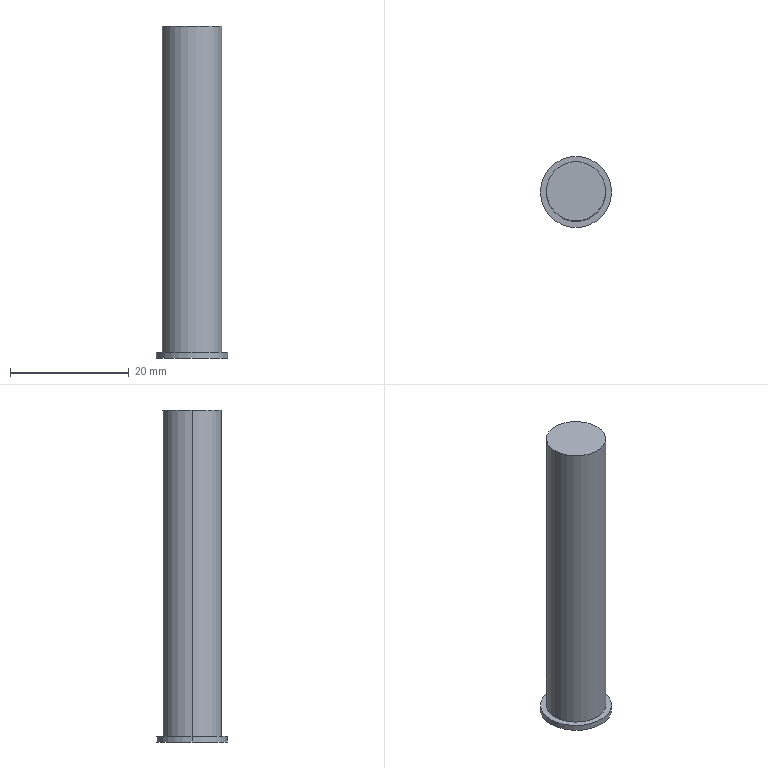Part | SolidWorks | features Extrusion 1, ICE 1 | 1 solid | 7 faces | box 12 x 12 x 56 mm | volume 4433 mm3 | cylinder 4 | plane 3 | commonest cylinder face diameters 10 x2 12 x2
STEP:
#1=CARTESIAN_POINT('',(-6.,0.,-1.));
#2=VERTEX_POINT('',#1);
#3=CARTESIAN_POINT('',(6.,0.,-1.));
#4=VERTEX_POINT('',#3);
#5=CARTESIAN_POINT('',(0.,0.,-1.));
#6=DIRECTION('',(0.,0.,-1.));
#7=DIRECTION('',(-1.,0.,0.));
#8=AXIS2_PLACEMENT_3D('',#5,#6,#7);
#9=CIRCLE('',#8,6.);
#10=EDGE_CURVE('',#2,#4,#9,.T.);
#11=ORIENTED_EDGE('',*,*,#10,.F.);
#12=CARTESIAN_POINT('',(-6.,0.,0.));
#13=VERTEX_POINT('',#12);
#14=CARTESIAN_POINT('',(-6.,0.,-1.));
#15=DIRECTION('',(0.,0.,1.));
#16=VECTOR('',#15,1000.);
#17=LINE('',#14,#16);
#18=EDGE_CURVE('',#2,#13,#17,.T.);
#19=ORIENTED_EDGE('',*,*,#18,.T.);
#20=CARTESIAN_POINT('',(6.,0.,0.));
#21=VERTEX_POINT('',#20);
#22=CARTESIAN_POINT('',(0.,0.,0.));
#23=DIRECTION('',(0.,0.,-1.));
#24=DIRECTION('',(-1.,0.,0.));
#25=AXIS2_PLACEMENT_3D('',#22,#23,#24);
#26=CIRCLE('',#25,6.);
#27=EDGE_CURVE('',#13,#21,#26,.T.);
#28=ORIENTED_EDGE('',*,*,#27,.T.);
#29=CARTESIAN_POINT('',(6.,0.,-1.));
#30=DIRECTION('',(0.,0.,1.));
#31=VECTOR('',#30,1000.);
#32=LINE('',#29,#31);
#33=EDGE_CURVE('',#4,#21,#32,.T.);
#34=ORIENTED_EDGE('',*,*,#33,.F.);
#35=EDGE_LOOP('',(#11,#19,#28,#34));
#36=FACE_OUTER_BOUND('',#35,.T.);
#37=CARTESIAN_POINT('',(0.,0.,-1.));
#38=DIRECTION('',(0.,0.,1.));
#39=DIRECTION('',(1.,0.,0.));
#40=AXIS2_PLACEMENT_3D('',#37,#38,#39);
#41=CYLINDRICAL_SURFACE('',#40,6.);
#42=ADVANCED_FACE('',(#36),#41,.T.);
#43=CARTESIAN_POINT('',(5.,0.,55.));
#44=VERTEX_POINT('',#43);
#45=CARTESIAN_POINT('',(-5.,0.,55.));
#46=VERTEX_POINT('',#45);
#47=CARTESIAN_POINT('',(0.,0.,55.));
#48=DIRECTION('',(0.,0.,1.));
#49=DIRECTION('',(1.,0.,0.));
#50=AXIS2_PLACEMENT_3D('',#47,#48,#49);
#51=CIRCLE('',#50,5.);
#52=EDGE_CURVE('',#44,#46,#51,.T.);
#53=ORIENTED_EDGE('',*,*,#52,.F.);
#54=CARTESIAN_POINT('',(5.,0.,0.));
#55=VERTEX_POINT('',#54);
#56=CARTESIAN_POINT('',(5.,0.,55.));
#57=DIRECTION('',(0.,0.,-1.));
#58=VECTOR('',#57,1000.);
#59=LINE('',#56,#58);
#60=EDGE_CURVE('',#44,#55,#59,.T.);
#61=ORIENTED_EDGE('',*,*,#60,.T.);
#62=CARTESIAN_POINT('',(-5.,0.,0.));
#63=VERTEX_POINT('',#62);
#64=CARTESIAN_POINT('',(0.,0.,0.));
#65=DIRECTION('',(0.,0.,1.));
#66=DIRECTION('',(1.,0.,0.));
#67=AXIS2_PLACEMENT_3D('',#64,#65,#66);
#68=CIRCLE('',#67,5.);
#69=EDGE_CURVE('',#55,#63,#68,.T.);
#70=ORIENTED_EDGE('',*,*,#69,.T.);
#71=CARTESIAN_POINT('',(-5.,0.,55.));
#72=DIRECTION('',(0.,0.,-1.));
#73=VECTOR('',#72,1000.);
#74=LINE('',#71,#73);
#75=EDGE_CURVE('',#46,#63,#74,.T.);
#76=ORIENTED_EDGE('',*,*,#75,.F.);
#77=EDGE_LOOP('',(#53,#61,#70,#76));
#78=FACE_OUTER_BOUND('',#77,.T.);
#79=CARTESIAN_POINT('',(0.,0.,55.));
#80=DIRECTION('',(0.,0.,-1.));
#81=DIRECTION('',(-1.,0.,0.));
#82=AXIS2_PLACEMENT_3D('',#79,#80,#81);
#83=CYLINDRICAL_SURFACE('',#82,5.);
#84=ADVANCED_FACE('',(#78),#83,.T.);
#85=ORIENTED_EDGE('',*,*,#60,.F.);
#86=CARTESIAN_POINT('',(0.,0.,55.));
#87=DIRECTION('',(0.,0.,1.));
#88=DIRECTION('',(1.,0.,0.));
#89=AXIS2_PLACEMENT_3D('',#86,#87,#88);
#90=CIRCLE('',#89,5.);
#91=EDGE_CURVE('',#46,#44,#90,.T.);
#92=ORIENTED_EDGE('',*,*,#91,.F.);
#93=ORIENTED_EDGE('',*,*,#75,.T.);
#94=CARTESIAN_POINT('',(0.,0.,0.));
#95=DIRECTION('',(0.,0.,1.));
#96=DIRECTION('',(1.,0.,0.));
#97=AXIS2_PLACEMENT_3D('',#94,#95,#96);
#98=CIRCLE('',#97,5.);
#99=EDGE_CURVE('',#63,#55,#98,.T.);
#100=ORIENTED_EDGE('',*,*,#99,.T.);
#101=EDGE_LOOP('',(#85,#92,#93,#100));
#102=FACE_OUTER_BOUND('',#101,.T.);
#103=CARTESIAN_POINT('',(0.,0.,55.));
#104=DIRECTION('',(0.,0.,-1.));
#105=DIRECTION('',(-1.,0.,0.));
#106=AXIS2_PLACEMENT_3D('',#103,#104,#105);
#107=CYLINDRICAL_SURFACE('',#106,5.);
#108=ADVANCED_FACE('',(#102),#107,.T.);
#109=ORIENTED_EDGE('',*,*,#91,.T.);
#110=ORIENTED_EDGE('',*,*,#52,.T.);
#111=EDGE_LOOP('',(#109,#110));
#112=FACE_OUTER_BOUND('',#111,.T.);
#113=CARTESIAN_POINT('',(0.,0.,55.));
#114=DIRECTION('',(0.,0.,1.));
#115=DIRECTION('',(1.,0.,0.));
#116=AXIS2_PLACEMENT_3D('',#113,#114,#115);
#117=PLANE('',#116);
#118=ADVANCED_FACE('',(#112),#117,.T.);
#119=ORIENTED_EDGE('',*,*,#18,.F.);
#120=CARTESIAN_POINT('',(0.,0.,-1.));
#121=DIRECTION('',(0.,0.,-1.));
#122=DIRECTION('',(-1.,0.,0.));
#123=AXIS2_PLACEMENT_3D('',#120,#121,#122);
#124=CIRCLE('',#123,6.);
#125=EDGE_CURVE('',#4,#2,#124,.T.);
#126=ORIENTED_EDGE('',*,*,#125,.F.);
#127=ORIENTED_EDGE('',*,*,#33,.T.);
#128=CARTESIAN_POINT('',(0.,0.,0.));
#129=DIRECTION('',(0.,0.,-1.));
#130=DIRECTION('',(-1.,0.,0.));
#131=AXIS2_PLACEMENT_3D('',#128,#129,#130);
#132=CIRCLE('',#131,6.);
#133=EDGE_CURVE('',#21,#13,#132,.T.);
#134=ORIENTED_EDGE('',*,*,#133,.T.);
#135=EDGE_LOOP('',(#119,#126,#127,#134));
#136=FACE_OUTER_BOUND('',#135,.T.);
#137=CARTESIAN_POINT('',(0.,0.,-1.));
#138=DIRECTION('',(0.,0.,1.));
#139=DIRECTION('',(1.,0.,0.));
#140=AXIS2_PLACEMENT_3D('',#137,#138,#139);
#141=CYLINDRICAL_SURFACE('',#140,6.);
#142=ADVANCED_FACE('',(#136),#141,.T.);
#143=ORIENTED_EDGE('',*,*,#125,.T.);
#144=ORIENTED_EDGE('',*,*,#10,.T.);
#145=EDGE_LOOP('',(#143,#144));
#146=FACE_OUTER_BOUND('',#145,.T.);
#147=CARTESIAN_POINT('',(0.,0.,-1.));
#148=DIRECTION('',(0.,0.,-1.));
#149=DIRECTION('',(-1.,0.,0.));
#150=AXIS2_PLACEMENT_3D('',#147,#148,#149);
#151=PLANE('',#150);
#152=ADVANCED_FACE('',(#146),#151,.T.);
#153=ORIENTED_EDGE('',*,*,#99,.F.);
#154=ORIENTED_EDGE('',*,*,#69,.F.);
#155=EDGE_LOOP('',(#153,#154));
#156=FACE_BOUND('',#155,.T.);
#157=ORIENTED_EDGE('',*,*,#133,.F.);
#158=ORIENTED_EDGE('',*,*,#27,.F.);
#159=EDGE_LOOP('',(#157,#158));
#160=FACE_OUTER_BOUND('',#159,.T.);
#161=CARTESIAN_POINT('',(0.,0.,0.));
#162=DIRECTION('',(0.,0.,-1.));
#163=DIRECTION('',(-1.,0.,0.));
#164=AXIS2_PLACEMENT_3D('',#161,#162,#163);
#165=PLANE('',#164);
#166=ADVANCED_FACE('',(#156,#160),#165,.F.);
#167=CLOSED_SHELL('',(#42,#84,#108,#118,#142,#152,#166));
#168=MANIFOLD_SOLID_BREP('',#167);
#169=CARTESIAN_POINT('',(0.,0.,0.));
#170=DIRECTION('',(0.,0.,1.));
#171=DIRECTION('',(1.,0.,0.));
#172=AXIS2_PLACEMENT_3D('',#169,#170,#171);
#173=(LENGTH_UNIT()NAMED_UNIT(*)SI_UNIT(.MILLI.,.METRE.));
#174=UNCERTAINTY_MEASURE_WITH_UNIT(LENGTH_MEASURE(0.00001),#173,'','');
#175=(NAMED_UNIT(*)PLANE_ANGLE_UNIT()SI_UNIT($,.RADIAN.));
#176=(NAMED_UNIT(*)SI_UNIT($,.STERADIAN.)SOLID_ANGLE_UNIT());
#177=(GEOMETRIC_REPRESENTATION_CONTEXT(3)GLOBAL_UNCERTAINTY_ASSIGNED_CONTEXT((#174))GLOBAL_UNIT_ASSIGNED_CONTEXT((#173,#175,#176))REPRESENTATION_CONTEXT('',''));
#178=ADVANCED_BREP_SHAPE_REPRESENTATION('',(#168,#172),#177);